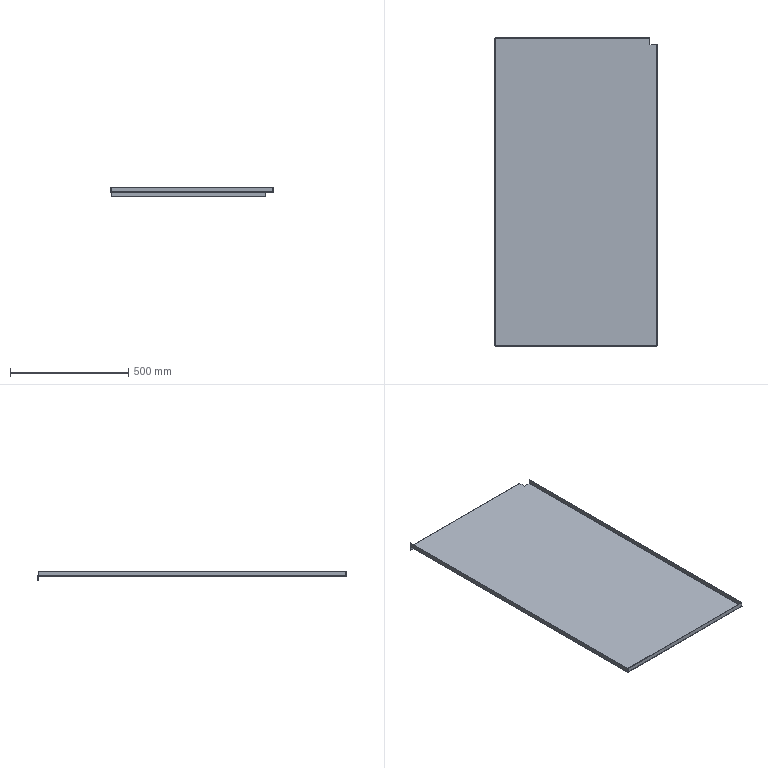Part | SolidWorks | 1 solid | 40 faces | box 685.001 x 1302 x 38.5 mm | volume 1442585 mm3 | plane 28 | cylinder 8 | spline 4 | commonest cylinder face diameters 0.2 x4 3.2 x4
STEP:
#1=CARTESIAN_POINT('',(342.5,621.,0.1));
#2=VERTEX_POINT('',#1);
#3=CARTESIAN_POINT('',(342.5,621.,18.5));
#4=VERTEX_POINT('',#3);
#5=CARTESIAN_POINT('',(342.5,621.,0.));
#6=DIRECTION('',(0.,0.,1.));
#7=VECTOR('',#6,1000.);
#8=LINE('',#5,#7);
#9=EDGE_CURVE('',#2,#4,#8,.T.);
#10=ORIENTED_EDGE('',*,*,#9,.F.);
#11=CARTESIAN_POINT('',(341.,621.,0.1));
#12=VERTEX_POINT('',#11);
#13=CARTESIAN_POINT('',(342.5,621.,0.1));
#14=DIRECTION('',(-1.,0.,0.));
#15=VECTOR('',#14,1000.);
#16=LINE('',#13,#15);
#17=EDGE_CURVE('',#2,#12,#16,.T.);
#18=ORIENTED_EDGE('',*,*,#17,.T.);
#19=CARTESIAN_POINT('',(341.,621.,18.5));
#20=VERTEX_POINT('',#19);
#21=CARTESIAN_POINT('',(341.,621.,0.));
#22=DIRECTION('',(0.,0.,1.));
#23=VECTOR('',#22,1000.);
#24=LINE('',#21,#23);
#25=EDGE_CURVE('',#12,#20,#24,.T.);
#26=ORIENTED_EDGE('',*,*,#25,.T.);
#27=CARTESIAN_POINT('',(362.5,621.,18.5));
#28=DIRECTION('',(1.,0.,0.));
#29=VECTOR('',#28,1000.);
#30=LINE('',#27,#29);
#31=EDGE_CURVE('',#20,#4,#30,.T.);
#32=ORIENTED_EDGE('',*,*,#31,.T.);
#33=EDGE_LOOP('',(#10,#18,#26,#32));
#34=FACE_OUTER_BOUND('',#33,.T.);
#35=CARTESIAN_POINT('',(362.5,621.,-20.));
#36=DIRECTION('',(0.,-1.,0.));
#37=DIRECTION('',(0.,0.,-1.));
#38=AXIS2_PLACEMENT_3D('',#35,#36,#37);
#39=PLANE('',#38);
#40=ADVANCED_FACE('',(#34),#39,.F.);
#41=CARTESIAN_POINT('',(312.5,621.,0.));
#42=VERTEX_POINT('',#41);
#43=CARTESIAN_POINT('',(340.9,621.,0.));
#44=VERTEX_POINT('',#43);
#45=CARTESIAN_POINT('',(0.,621.,0.));
#46=DIRECTION('',(1.,0.,0.));
#47=VECTOR('',#46,1000.);
#48=LINE('',#45,#47);
#49=EDGE_CURVE('',#42,#44,#48,.T.);
#50=ORIENTED_EDGE('',*,*,#49,.T.);
#51=CARTESIAN_POINT('',(340.9,621.,-1.5));
#52=VERTEX_POINT('',#51);
#53=CARTESIAN_POINT('',(340.9,621.,0.));
#54=DIRECTION('',(0.,0.,-1.));
#55=VECTOR('',#54,1000.);
#56=LINE('',#53,#55);
#57=EDGE_CURVE('',#44,#52,#56,.T.);
#58=ORIENTED_EDGE('',*,*,#57,.T.);
#59=CARTESIAN_POINT('',(312.5,621.,-1.5));
#60=VERTEX_POINT('',#59);
#61=CARTESIAN_POINT('',(0.,621.,-1.5));
#62=DIRECTION('',(1.,0.,0.));
#63=VECTOR('',#62,1000.);
#64=LINE('',#61,#63);
#65=EDGE_CURVE('',#60,#52,#64,.T.);
#66=ORIENTED_EDGE('',*,*,#65,.F.);
#67=CARTESIAN_POINT('',(312.5,621.,-20.));
#68=DIRECTION('',(0.,0.,1.));
#69=VECTOR('',#68,1000.);
#70=LINE('',#67,#69);
#71=EDGE_CURVE('',#60,#42,#70,.T.);
#72=ORIENTED_EDGE('',*,*,#71,.T.);
#73=EDGE_LOOP('',(#50,#58,#66,#72));
#74=FACE_OUTER_BOUND('',#73,.T.);
#75=CARTESIAN_POINT('',(362.5,621.,-20.));
#76=DIRECTION('',(0.,-1.,0.));
#77=DIRECTION('',(0.,0.,-1.));
#78=AXIS2_PLACEMENT_3D('',#75,#76,#77);
#79=PLANE('',#78);
#80=ADVANCED_FACE('',(#74),#79,.F.);
#81=CARTESIAN_POINT('',(312.5,651.,-20.));
#82=VERTEX_POINT('',#81);
#83=CARTESIAN_POINT('',(312.5,651.,-1.6));
#84=VERTEX_POINT('',#83);
#85=CARTESIAN_POINT('',(312.5,651.,0.));
#86=DIRECTION('',(0.,0.,1.));
#87=VECTOR('',#86,1000.);
#88=LINE('',#85,#87);
#89=EDGE_CURVE('',#82,#84,#88,.T.);
#90=ORIENTED_EDGE('',*,*,#89,.T.);
#91=CARTESIAN_POINT('',(312.5,649.5,-1.6));
#92=VERTEX_POINT('',#91);
#93=CARTESIAN_POINT('',(312.5,651.,-1.6));
#94=DIRECTION('',(0.,-1.,0.));
#95=VECTOR('',#94,1000.);
#96=LINE('',#93,#95);
#97=EDGE_CURVE('',#84,#92,#96,.T.);
#98=ORIENTED_EDGE('',*,*,#97,.T.);
#99=CARTESIAN_POINT('',(312.5,649.5,-20.));
#100=VERTEX_POINT('',#99);
#101=CARTESIAN_POINT('',(312.5,649.5,0.));
#102=DIRECTION('',(0.,0.,1.));
#103=VECTOR('',#102,1000.);
#104=LINE('',#101,#103);
#105=EDGE_CURVE('',#100,#92,#104,.T.);
#106=ORIENTED_EDGE('',*,*,#105,.F.);
#107=CARTESIAN_POINT('',(312.5,621.,-20.));
#108=DIRECTION('',(0.,-1.,0.));
#109=VECTOR('',#108,1000.);
#110=LINE('',#107,#109);
#111=EDGE_CURVE('',#82,#100,#110,.T.);
#112=ORIENTED_EDGE('',*,*,#111,.F.);
#113=EDGE_LOOP('',(#90,#98,#106,#112));
#114=FACE_OUTER_BOUND('',#113,.T.);
#115=CARTESIAN_POINT('',(312.5,621.,-20.));
#116=DIRECTION('',(-1.,0.,0.));
#117=DIRECTION('',(0.,0.,1.));
#118=AXIS2_PLACEMENT_3D('',#115,#116,#117);
#119=PLANE('',#118);
#120=ADVANCED_FACE('',(#114),#119,.F.);
#121=CARTESIAN_POINT('',(312.5,649.4,-1.5));
#122=VERTEX_POINT('',#121);
#123=CARTESIAN_POINT('',(312.5,0.,-1.5));
#124=DIRECTION('',(0.,-1.,0.));
#125=VECTOR('',#124,1000.);
#126=LINE('',#123,#125);
#127=EDGE_CURVE('',#122,#60,#126,.T.);
#128=ORIENTED_EDGE('',*,*,#127,.F.);
#129=CARTESIAN_POINT('',(312.5,649.4,0.));
#130=VERTEX_POINT('',#129);
#131=CARTESIAN_POINT('',(312.5,649.4,-1.5));
#132=DIRECTION('',(0.,0.,1.));
#133=VECTOR('',#132,1000.);
#134=LINE('',#131,#133);
#135=EDGE_CURVE('',#122,#130,#134,.T.);
#136=ORIENTED_EDGE('',*,*,#135,.T.);
#137=CARTESIAN_POINT('',(312.5,0.,0.));
#138=DIRECTION('',(0.,-1.,0.));
#139=VECTOR('',#138,1000.);
#140=LINE('',#137,#139);
#141=EDGE_CURVE('',#130,#42,#140,.T.);
#142=ORIENTED_EDGE('',*,*,#141,.T.);
#143=ORIENTED_EDGE('',*,*,#71,.F.);
#144=EDGE_LOOP('',(#128,#136,#142,#143));
#145=FACE_OUTER_BOUND('',#144,.T.);
#146=CARTESIAN_POINT('',(312.5,621.,-20.));
#147=DIRECTION('',(-1.,0.,0.));
#148=DIRECTION('',(0.,0.,1.));
#149=AXIS2_PLACEMENT_3D('',#146,#147,#148);
#150=PLANE('',#149);
#151=ADVANCED_FACE('',(#145),#150,.F.);
#152=ORIENTED_EDGE('',*,*,#127,.T.);
#153=ORIENTED_EDGE('',*,*,#65,.T.);
#154=CARTESIAN_POINT('',(340.9,-649.4,-1.5));
#155=VERTEX_POINT('',#154);
#156=CARTESIAN_POINT('',(340.9,649.4,-1.5));
#157=DIRECTION('',(0.,-1.,0.));
#158=VECTOR('',#157,1000.);
#159=LINE('',#156,#158);
#160=EDGE_CURVE('',#52,#155,#159,.T.);
#161=ORIENTED_EDGE('',*,*,#160,.T.);
#162=CARTESIAN_POINT('',(-340.9,-649.4,-1.5));
#163=VERTEX_POINT('',#162);
#164=CARTESIAN_POINT('',(340.9,-649.4,-1.5));
#165=DIRECTION('',(-1.,0.,0.));
#166=VECTOR('',#165,1000.);
#167=LINE('',#164,#166);
#168=EDGE_CURVE('',#155,#163,#167,.T.);
#169=ORIENTED_EDGE('',*,*,#168,.T.);
#170=CARTESIAN_POINT('',(-340.9,649.4,-1.5));
#171=VERTEX_POINT('',#170);
#172=CARTESIAN_POINT('',(-340.9,-649.4,-1.5));
#173=DIRECTION('',(0.,1.,0.));
#174=VECTOR('',#173,1000.);
#175=LINE('',#172,#174);
#176=EDGE_CURVE('',#163,#171,#175,.T.);
#177=ORIENTED_EDGE('',*,*,#176,.T.);
#178=CARTESIAN_POINT('',(340.9,649.4,-1.5));
#179=DIRECTION('',(-1.,0.,0.));
#180=VECTOR('',#179,1000.);
#181=LINE('',#178,#180);
#182=EDGE_CURVE('',#122,#171,#181,.T.);
#183=ORIENTED_EDGE('',*,*,#182,.F.);
#184=EDGE_LOOP('',(#152,#153,#161,#169,#177,#183));
#185=FACE_OUTER_BOUND('',#184,.T.);
#186=CARTESIAN_POINT('',(0.,0.,-1.5));
#187=DIRECTION('',(0.,0.,1.));
#188=DIRECTION('',(1.,0.,0.));
#189=AXIS2_PLACEMENT_3D('',#186,#187,#188);
#190=PLANE('',#189);
#191=ADVANCED_FACE('',(#185),#190,.F.);
#192=ORIENTED_EDGE('',*,*,#49,.F.);
#193=ORIENTED_EDGE('',*,*,#141,.F.);
#194=CARTESIAN_POINT('',(-340.9,649.4,0.));
#195=VERTEX_POINT('',#194);
#196=CARTESIAN_POINT('',(340.9,649.4,0.));
#197=DIRECTION('',(-1.,0.,0.));
#198=VECTOR('',#197,1000.);
#199=LINE('',#196,#198);
#200=EDGE_CURVE('',#130,#195,#199,.T.);
#201=ORIENTED_EDGE('',*,*,#200,.T.);
#202=CARTESIAN_POINT('',(-340.9,-649.4,0.));
#203=VERTEX_POINT('',#202);
#204=CARTESIAN_POINT('',(-340.9,-649.4,0.));
#205=DIRECTION('',(0.,1.,0.));
#206=VECTOR('',#205,1000.);
#207=LINE('',#204,#206);
#208=EDGE_CURVE('',#203,#195,#207,.T.);
#209=ORIENTED_EDGE('',*,*,#208,.F.);
#210=CARTESIAN_POINT('',(340.9,-649.4,0.));
#211=VERTEX_POINT('',#210);
#212=CARTESIAN_POINT('',(340.9,-649.4,0.));
#213=DIRECTION('',(-1.,0.,0.));
#214=VECTOR('',#213,1000.);
#215=LINE('',#212,#214);
#216=EDGE_CURVE('',#211,#203,#215,.T.);
#217=ORIENTED_EDGE('',*,*,#216,.F.);
#218=CARTESIAN_POINT('',(340.9,649.4,0.));
#219=DIRECTION('',(0.,-1.,0.));
#220=VECTOR('',#219,1000.);
#221=LINE('',#218,#220);
#222=EDGE_CURVE('',#44,#211,#221,.T.);
#223=ORIENTED_EDGE('',*,*,#222,.F.);
#224=EDGE_LOOP('',(#192,#193,#201,#209,#217,#223));
#225=FACE_OUTER_BOUND('',#224,.T.);
#226=CARTESIAN_POINT('',(0.,0.,0.));
#227=DIRECTION('',(0.,0.,1.));
#228=DIRECTION('',(1.,0.,0.));
#229=AXIS2_PLACEMENT_3D('',#226,#227,#228);
#230=PLANE('',#229);
#231=ADVANCED_FACE('',(#225),#230,.T.);
#232=CARTESIAN_POINT('',(-342.5,649.4,0.1));
#233=VERTEX_POINT('',#232);
#234=CARTESIAN_POINT('',(-341.,649.4,0.1));
#235=VERTEX_POINT('',#234);
#236=CARTESIAN_POINT('',(-341.,649.4,0.1));
#237=DIRECTION('',(1.,0.,0.));
#238=VECTOR('',#237,1000.);
#239=LINE('',#236,#238);
#240=EDGE_CURVE('',#233,#235,#239,.T.);
#241=ORIENTED_EDGE('',*,*,#240,.T.);
#242=CARTESIAN_POINT('',(-340.9,649.4,0.1));
#243=DIRECTION('',(0.,1.,0.));
#244=DIRECTION('',(0.,0.,-1.));
#245=AXIS2_PLACEMENT_3D('',#242,#243,#244);
#246=CIRCLE('',#245,0.1);
#247=EDGE_CURVE('',#195,#235,#246,.T.);
#248=ORIENTED_EDGE('',*,*,#247,.F.);
#249=CARTESIAN_POINT('',(-340.9,649.4,0.));
#250=DIRECTION('',(0.,0.,-1.));
#251=VECTOR('',#250,1000.);
#252=LINE('',#249,#251);
#253=EDGE_CURVE('',#195,#171,#252,.T.);
#254=ORIENTED_EDGE('',*,*,#253,.T.);
#255=CARTESIAN_POINT('',(-340.9,649.4,0.1));
#256=DIRECTION('',(0.,1.,0.));
#257=DIRECTION('',(0.,0.,-1.));
#258=AXIS2_PLACEMENT_3D('',#255,#256,#257);
#259=CIRCLE('',#258,1.6);
#260=EDGE_CURVE('',#171,#233,#259,.T.);
#261=ORIENTED_EDGE('',*,*,#260,.T.);
#262=EDGE_LOOP('',(#241,#248,#254,#261));
#263=FACE_OUTER_BOUND('',#262,.T.);
#264=CARTESIAN_POINT('',(-340.9,649.4,0.1));
#265=DIRECTION('',(0.,1.,0.));
#266=DIRECTION('',(0.,0.,1.));
#267=AXIS2_PLACEMENT_3D('',#264,#265,#266);
#268=PLANE('',#267);
#269=ADVANCED_FACE('',(#263),#268,.T.);
#270=CARTESIAN_POINT('',(-341.,-648.793,0.1));
#271=VERTEX_POINT('',#270);
#272=CARTESIAN_POINT('',(-341.,-648.793,0.1));
#273=CARTESIAN_POINT('',(-341.,-648.894,0.07382));
#274=CARTESIAN_POINT('',(-340.989,-648.995,0.0478));
#275=CARTESIAN_POINT('',(-340.952,-649.198,0.01078));
#276=CARTESIAN_POINT('',(-340.926,-649.299,0.));
#277=CARTESIAN_POINT('',(-340.9,-649.4,0.));
#278=B_SPLINE_CURVE_WITH_KNOTS('',3,(#272,#273,#274,#275,#276,#277),.UNSPECIFIED.,.F.,.F.,(4,2,4),(0.,0.5,1.),.UNSPECIFIED.);
#279=EDGE_CURVE('',#271,#203,#278,.T.);
#280=ORIENTED_EDGE('',*,*,#279,.F.);
#281=CARTESIAN_POINT('',(-342.5,-648.793,0.1));
#282=VERTEX_POINT('',#281);
#283=CARTESIAN_POINT('',(-341.,-648.793,0.1));
#284=DIRECTION('',(1.,0.,0.));
#285=VECTOR('',#284,1000.);
#286=LINE('',#283,#285);
#287=EDGE_CURVE('',#282,#271,#286,.T.);
#288=ORIENTED_EDGE('',*,*,#287,.F.);
#289=CARTESIAN_POINT('',(-342.5,-648.793,0.1));
#290=CARTESIAN_POINT('',(-342.5,-648.844,-0.1115));
#291=CARTESIAN_POINT('',(-342.46,-648.893,-0.3151));
#292=CARTESIAN_POINT('',(-342.299,-648.995,-0.7048));
#293=CARTESIAN_POINT('',(-342.181,-649.045,-0.881));
#294=CARTESIAN_POINT('',(-341.958,-649.121,-1.105));
#295=CARTESIAN_POINT('',(-341.878,-649.147,-1.171));
#296=CARTESIAN_POINT('',(-341.704,-649.197,-1.287));
#297=CARTESIAN_POINT('',(-341.61,-649.223,-1.338));
#298=CARTESIAN_POINT('',(-341.32,-649.299,-1.458));
#299=CARTESIAN_POINT('',(-341.112,-649.349,-1.5));
#300=CARTESIAN_POINT('',(-340.9,-649.4,-1.5));
#301=B_SPLINE_CURVE_WITH_KNOTS('',3,(#289,#290,#291,#292,#293,#294,#295,#296,#297,#298,#299,#300),.UNSPECIFIED.,.F.,.F.,(4,2,2,2,2,4),(0.,0.0006399,0.00128,0.0016,0.00192,0.00256),.UNSPECIFIED.);
#302=EDGE_CURVE('',#282,#163,#301,.T.);
#303=ORIENTED_EDGE('',*,*,#302,.T.);
#304=CARTESIAN_POINT('',(-340.9,-649.4,0.));
#305=DIRECTION('',(0.,0.,-1.));
#306=VECTOR('',#305,1000.);
#307=LINE('',#304,#306);
#308=EDGE_CURVE('',#203,#163,#307,.T.);
#309=ORIENTED_EDGE('',*,*,#308,.F.);
#310=EDGE_LOOP('',(#280,#288,#303,#309));
#311=FACE_OUTER_BOUND('',#310,.T.);
#312=CARTESIAN_POINT('',(-342.515,-648.793,0.1));
#313=CARTESIAN_POINT('',(-342.515,-648.843,-0.1114));
#314=CARTESIAN_POINT('',(-342.473,-648.894,-0.3227));
#315=CARTESIAN_POINT('',(-342.311,-648.995,-0.7133));
#316=CARTESIAN_POINT('',(-342.191,-649.046,-0.8925));
#317=CARTESIAN_POINT('',(-341.892,-649.147,-1.191));
#318=CARTESIAN_POINT('',(-341.713,-649.198,-1.311));
#319=CARTESIAN_POINT('',(-341.323,-649.299,-1.473));
#320=CARTESIAN_POINT('',(-341.111,-649.349,-1.515));
#321=CARTESIAN_POINT('',(-340.9,-649.4,-1.515));
#322=CARTESIAN_POINT('',(-342.5,-648.793,0.1));
#323=CARTESIAN_POINT('',(-342.5,-648.843,-0.1095));
#324=CARTESIAN_POINT('',(-342.458,-648.894,-0.3188));
#325=CARTESIAN_POINT('',(-342.298,-648.995,-0.7058));
#326=CARTESIAN_POINT('',(-342.179,-649.046,-0.8833));
#327=CARTESIAN_POINT('',(-341.883,-649.147,-1.179));
#328=CARTESIAN_POINT('',(-341.706,-649.198,-1.298));
#329=CARTESIAN_POINT('',(-341.319,-649.299,-1.458));
#330=CARTESIAN_POINT('',(-341.109,-649.349,-1.5));
#331=CARTESIAN_POINT('',(-340.9,-649.4,-1.5));
#332=CARTESIAN_POINT('',(-341.,-648.793,0.1));
#333=CARTESIAN_POINT('',(-341.,-648.843,0.08691));
#334=CARTESIAN_POINT('',(-340.997,-648.894,0.07383));
#335=CARTESIAN_POINT('',(-340.987,-648.995,0.04964));
#336=CARTESIAN_POINT('',(-340.98,-649.046,0.03855));
#337=CARTESIAN_POINT('',(-340.961,-649.147,0.02003));
#338=CARTESIAN_POINT('',(-340.95,-649.198,0.01262));
#339=CARTESIAN_POINT('',(-340.926,-649.299,0.002603));
#340=CARTESIAN_POINT('',(-340.913,-649.349,0.));
#341=CARTESIAN_POINT('',(-340.9,-649.4,0.));
#342=B_SPLINE_SURFACE_WITH_KNOTS('',1,3,((#312,#313,#314,#315,#316,#317,#318,#319,#320,#321),(#322,#323,#324,#325,#326,#327,#328,#329,#330,#331),(#332,#333,#334,#335,#336,#337,#338,#339,#340,#341)),.UNSPECIFIED.,.F.,.F.,.F.,(2,1,2),(4,2,2,2,4),(-0.01,0.,1.),(0.,0.25,0.5,0.75,1.),.UNSPECIFIED.);
#343=ADVANCED_FACE('',(#311),#342,.F.);
#344=ORIENTED_EDGE('',*,*,#176,.F.);
#345=ORIENTED_EDGE('',*,*,#302,.F.);
#346=CARTESIAN_POINT('',(-342.5,651.,0.1));
#347=DIRECTION('',(0.,1.,0.));
#348=VECTOR('',#347,1000.);
#349=LINE('',#346,#348);
#350=EDGE_CURVE('',#282,#233,#349,.T.);
#351=ORIENTED_EDGE('',*,*,#350,.T.);
#352=ORIENTED_EDGE('',*,*,#260,.F.);
#353=EDGE_LOOP('',(#344,#345,#351,#352));
#354=FACE_OUTER_BOUND('',#353,.T.);
#355=CARTESIAN_POINT('',(-340.9,-649.4,0.1));
#356=DIRECTION('',(0.,-1.,0.));
#357=DIRECTION('',(-1.,0.,0.));
#358=AXIS2_PLACEMENT_3D('',#355,#356,#357);
#359=CYLINDRICAL_SURFACE('',#358,1.6);
#360=ADVANCED_FACE('',(#354),#359,.T.);
#361=ORIENTED_EDGE('',*,*,#208,.T.);
#362=ORIENTED_EDGE('',*,*,#247,.T.);
#363=CARTESIAN_POINT('',(-341.,651.,0.1));
#364=DIRECTION('',(0.,-1.,0.));
#365=VECTOR('',#364,1000.);
#366=LINE('',#363,#365);
#367=EDGE_CURVE('',#235,#271,#366,.T.);
#368=ORIENTED_EDGE('',*,*,#367,.T.);
#369=ORIENTED_EDGE('',*,*,#279,.T.);
#370=EDGE_LOOP('',(#361,#362,#368,#369));
#371=FACE_OUTER_BOUND('',#370,.T.);
#372=CARTESIAN_POINT('',(-340.9,-649.4,0.1));
#373=DIRECTION('',(0.,-1.,0.));
#374=DIRECTION('',(-1.,0.,0.));
#375=AXIS2_PLACEMENT_3D('',#372,#373,#374);
#376=CYLINDRICAL_SURFACE('',#375,0.1);
#377=ADVANCED_FACE('',(#371),#376,.F.);
#378=CARTESIAN_POINT('',(-342.5,649.4,18.5));
#379=VERTEX_POINT('',#378);
#380=CARTESIAN_POINT('',(-342.5,649.4,0.));
#381=DIRECTION('',(0.,0.,1.));
#382=VECTOR('',#381,1000.);
#383=LINE('',#380,#382);
#384=EDGE_CURVE('',#233,#379,#383,.T.);
#385=ORIENTED_EDGE('',*,*,#384,.T.);
#386=CARTESIAN_POINT('',(-341.,649.4,18.5));
#387=VERTEX_POINT('',#386);
#388=CARTESIAN_POINT('',(-341.,649.4,18.5));
#389=DIRECTION('',(1.,0.,0.));
#390=VECTOR('',#389,1000.);
#391=LINE('',#388,#390);
#392=EDGE_CURVE('',#379,#387,#391,.T.);
#393=ORIENTED_EDGE('',*,*,#392,.T.);
#394=CARTESIAN_POINT('',(-341.,649.4,0.));
#395=DIRECTION('',(0.,0.,1.));
#396=VECTOR('',#395,1000.);
#397=LINE('',#394,#396);
#398=EDGE_CURVE('',#235,#387,#397,.T.);
#399=ORIENTED_EDGE('',*,*,#398,.F.);
#400=ORIENTED_EDGE('',*,*,#240,.F.);
#401=EDGE_LOOP('',(#385,#393,#399,#400));
#402=FACE_OUTER_BOUND('',#401,.T.);
#403=CARTESIAN_POINT('',(-341.,649.4,0.));
#404=DIRECTION('',(0.,1.,0.));
#405=DIRECTION('',(0.,0.,1.));
#406=AXIS2_PLACEMENT_3D('',#403,#404,#405);
#407=PLANE('',#406);
#408=ADVANCED_FACE('',(#402),#407,.T.);
#409=ORIENTED_EDGE('',*,*,#350,.F.);
#410=CARTESIAN_POINT('',(-342.5,-648.793,18.5));
#411=VERTEX_POINT('',#410);
#412=CARTESIAN_POINT('',(-342.5,-648.793,0.));
#413=DIRECTION('',(0.,0.,1.));
#414=VECTOR('',#413,1000.);
#415=LINE('',#412,#414);
#416=EDGE_CURVE('',#282,#411,#415,.T.);
#417=ORIENTED_EDGE('',*,*,#416,.T.);
#418=CARTESIAN_POINT('',(-342.5,0.,18.5));
#419=DIRECTION('',(0.,1.,0.));
#420=VECTOR('',#419,1000.);
#421=LINE('',#418,#420);
#422=EDGE_CURVE('',#411,#379,#421,.T.);
#423=ORIENTED_EDGE('',*,*,#422,.T.);
#424=ORIENTED_EDGE('',*,*,#384,.F.);
#425=EDGE_LOOP('',(#409,#417,#423,#424));
#426=FACE_OUTER_BOUND('',#425,.T.);
#427=CARTESIAN_POINT('',(-342.5,0.,0.));
#428=DIRECTION('',(1.,0.,0.));
#429=DIRECTION('',(0.,0.,-1.));
#430=AXIS2_PLACEMENT_3D('',#427,#428,#429);
#431=PLANE('',#430);
#432=ADVANCED_FACE('',(#426),#431,.F.);
#433=CARTESIAN_POINT('',(-341.,-648.793,18.5));
#434=VERTEX_POINT('',#433);
#435=CARTESIAN_POINT('',(-341.,-648.793,0.));
#436=DIRECTION('',(0.,0.,1.));
#437=VECTOR('',#436,1000.);
#438=LINE('',#435,#437);
#439=EDGE_CURVE('',#271,#434,#438,.T.);
#440=ORIENTED_EDGE('',*,*,#439,.F.);
#441=ORIENTED_EDGE('',*,*,#367,.F.);
#442=ORIENTED_EDGE('',*,*,#398,.T.);
#443=CARTESIAN_POINT('',(-341.,651.,18.5));
#444=DIRECTION('',(0.,1.,0.));
#445=VECTOR('',#444,1000.);
#446=LINE('',#443,#445);
#447=EDGE_CURVE('',#434,#387,#446,.T.);
#448=ORIENTED_EDGE('',*,*,#447,.F.);
#449=EDGE_LOOP('',(#440,#441,#442,#448));
#450=FACE_OUTER_BOUND('',#449,.T.);
#451=CARTESIAN_POINT('',(-341.,0.,0.));
#452=DIRECTION('',(1.,0.,0.));
#453=DIRECTION('',(0.,0.,-1.));
#454=AXIS2_PLACEMENT_3D('',#451,#452,#453);
#455=PLANE('',#454);
#456=ADVANCED_FACE('',(#450),#455,.T.);
#457=ORIENTED_EDGE('',*,*,#422,.F.);
#458=CARTESIAN_POINT('',(-342.5,-648.793,18.5));
#459=DIRECTION('',(1.,0.,0.));
#460=VECTOR('',#459,1000.);
#461=LINE('',#458,#460);
#462=EDGE_CURVE('',#411,#434,#461,.T.);
#463=ORIENTED_EDGE('',*,*,#462,.T.);
#464=ORIENTED_EDGE('',*,*,#447,.T.);
#465=ORIENTED_EDGE('',*,*,#392,.F.);
#466=EDGE_LOOP('',(#457,#463,#464,#465));
#467=FACE_OUTER_BOUND('',#466,.T.);
#468=CARTESIAN_POINT('',(-342.5,651.,18.5));
#469=DIRECTION('',(0.,0.,-1.));
#470=DIRECTION('',(-1.,0.,0.));
#471=AXIS2_PLACEMENT_3D('',#468,#469,#470);
#472=PLANE('',#471);
#473=ADVANCED_FACE('',(#467),#472,.F.);
#474=ORIENTED_EDGE('',*,*,#462,.F.);
#475=ORIENTED_EDGE('',*,*,#416,.F.);
#476=ORIENTED_EDGE('',*,*,#287,.T.);
#477=ORIENTED_EDGE('',*,*,#439,.T.);
#478=EDGE_LOOP('',(#474,#475,#476,#477));
#479=FACE_OUTER_BOUND('',#478,.T.);
#480=CARTESIAN_POINT('',(-341.,-648.793,0.));
#481=DIRECTION('',(0.,1.,0.));
#482=DIRECTION('',(0.,0.,1.));
#483=AXIS2_PLACEMENT_3D('',#480,#481,#482);
#484=PLANE('',#483);
#485=ADVANCED_FACE('',(#479),#484,.F.);
#486=CARTESIAN_POINT('',(-340.9,651.,-1.6));
#487=VERTEX_POINT('',#486);
#488=CARTESIAN_POINT('',(-340.9,649.5,-1.6));
#489=VERTEX_POINT('',#488);
#490=CARTESIAN_POINT('',(-340.9,649.5,-1.6));
#491=DIRECTION('',(0.,-1.,0.));
#492=VECTOR('',#491,1000.);
#493=LINE('',#490,#492);
#494=EDGE_CURVE('',#487,#489,#493,.T.);
#495=ORIENTED_EDGE('',*,*,#494,.T.);
#496=CARTESIAN_POINT('',(-340.9,649.4,-1.6));
#497=DIRECTION('',(-1.,0.,0.));
#498=DIRECTION('',(0.,0.,-1.));
#499=AXIS2_PLACEMENT_3D('',#496,#497,#498);
#500=CIRCLE('',#499,0.1);
#501=EDGE_CURVE('',#171,#489,#500,.T.);
#502=ORIENTED_EDGE('',*,*,#501,.F.);
#503=ORIENTED_EDGE('',*,*,#253,.F.);
#504=CARTESIAN_POINT('',(-340.9,649.4,-1.6));
#505=DIRECTION('',(-1.,0.,0.));
#506=DIRECTION('',(0.,0.,-1.));
#507=AXIS2_PLACEMENT_3D('',#504,#505,#506);
#508=CIRCLE('',#507,1.6);
#509=EDGE_CURVE('',#195,#487,#508,.T.);
#510=ORIENTED_EDGE('',*,*,#509,.T.);
#511=EDGE_LOOP('',(#495,#502,#503,#510));
#512=FACE_OUTER_BOUND('',#511,.T.);
#513=CARTESIAN_POINT('',(-340.9,649.4,-1.6));
#514=DIRECTION('',(-1.,0.,0.));
#515=DIRECTION('',(0.,0.,1.));
#516=AXIS2_PLACEMENT_3D('',#513,#514,#515);
#517=PLANE('',#516);
#518=ADVANCED_FACE('',(#512),#517,.T.);
#519=CARTESIAN_POINT('',(312.5,649.4,-1.6));
#520=DIRECTION('',(1.,0.,0.));
#521=DIRECTION('',(0.,0.,1.));
#522=AXIS2_PLACEMENT_3D('',#519,#520,#521);
#523=CIRCLE('',#522,1.6);
#524=EDGE_CURVE('',#84,#130,#523,.T.);
#525=ORIENTED_EDGE('',*,*,#524,.F.);
#526=CARTESIAN_POINT('',(0.,651.,-1.6));
#527=DIRECTION('',(1.,0.,0.));
#528=VECTOR('',#527,1000.);
#529=LINE('',#526,#528);
#530=EDGE_CURVE('',#487,#84,#529,.T.);
#531=ORIENTED_EDGE('',*,*,#530,.F.);
#532=ORIENTED_EDGE('',*,*,#509,.F.);
#533=ORIENTED_EDGE('',*,*,#200,.F.);
#534=EDGE_LOOP('',(#525,#531,#532,#533));
#535=FACE_OUTER_BOUND('',#534,.T.);
#536=CARTESIAN_POINT('',(340.9,649.4,-1.6));
#537=DIRECTION('',(1.,0.,0.));
#538=DIRECTION('',(0.,1.,0.));
#539=AXIS2_PLACEMENT_3D('',#536,#537,#538);
#540=CYLINDRICAL_SURFACE('',#539,1.6);
#541=ADVANCED_FACE('',(#535),#540,.T.);
#542=CARTESIAN_POINT('',(-342.5,649.5,-1.6));
#543=DIRECTION('',(1.,0.,0.));
#544=VECTOR('',#543,1000.);
#545=LINE('',#542,#544);
#546=EDGE_CURVE('',#489,#92,#545,.T.);
#547=ORIENTED_EDGE('',*,*,#546,.T.);
#548=CARTESIAN_POINT('',(312.5,649.4,-1.6));
#549=DIRECTION('',(1.,0.,0.));
#550=DIRECTION('',(0.,0.,1.));
#551=AXIS2_PLACEMENT_3D('',#548,#549,#550);
#552=CIRCLE('',#551,0.1);
#553=EDGE_CURVE('',#92,#122,#552,.T.);
#554=ORIENTED_EDGE('',*,*,#553,.T.);
#555=ORIENTED_EDGE('',*,*,#182,.T.);
#556=ORIENTED_EDGE('',*,*,#501,.T.);
#557=EDGE_LOOP('',(#547,#554,#555,#556));
#558=FACE_OUTER_BOUND('',#557,.T.);
#559=CARTESIAN_POINT('',(340.9,649.4,-1.6));
#560=DIRECTION('',(1.,0.,0.));
#561=DIRECTION('',(0.,1.,0.));
#562=AXIS2_PLACEMENT_3D('',#559,#560,#561);
#563=CYLINDRICAL_SURFACE('',#562,0.1);
#564=ADVANCED_FACE('',(#558),#563,.F.);
#565=CARTESIAN_POINT('',(-340.9,649.5,-20.));
#566=VERTEX_POINT('',#565);
#567=CARTESIAN_POINT('',(-340.9,651.,-20.));
#568=VERTEX_POINT('',#567);
#569=CARTESIAN_POINT('',(-340.9,651.,-20.));
#570=DIRECTION('',(0.,1.,0.));
#571=VECTOR('',#570,1000.);
#572=LINE('',#569,#571);
#573=EDGE_CURVE('',#566,#568,#572,.T.);
#574=ORIENTED_EDGE('',*,*,#573,.F.);
#575=CARTESIAN_POINT('',(-340.9,649.5,0.));
#576=DIRECTION('',(0.,0.,-1.));
#577=VECTOR('',#576,1000.);
#578=LINE('',#575,#577);
#579=EDGE_CURVE('',#489,#566,#578,.T.);
#580=ORIENTED_EDGE('',*,*,#579,.F.);
#581=ORIENTED_EDGE('',*,*,#494,.F.);
#582=CARTESIAN_POINT('',(-340.9,651.,0.));
#583=DIRECTION('',(0.,0.,1.));
#584=VECTOR('',#583,1000.);
#585=LINE('',#582,#584);
#586=EDGE_CURVE('',#568,#487,#585,.T.);
#587=ORIENTED_EDGE('',*,*,#586,.F.);
#588=EDGE_LOOP('',(#574,#580,#581,#587));
#589=FACE_OUTER_BOUND('',#588,.T.);
#590=CARTESIAN_POINT('',(-340.9,649.5,-1.5));
#591=DIRECTION('',(-1.,0.,0.));
#592=DIRECTION('',(0.,0.,1.));
#593=AXIS2_PLACEMENT_3D('',#590,#591,#592);
#594=PLANE('',#593);
#595=ADVANCED_FACE('',(#589),#594,.T.);
#596=ORIENTED_EDGE('',*,*,#89,.F.);
#597=CARTESIAN_POINT('',(342.5,651.,-20.));
#598=DIRECTION('',(1.,0.,0.));
#599=VECTOR('',#598,1000.);
#600=LINE('',#597,#599);
#601=EDGE_CURVE('',#568,#82,#600,.T.);
#602=ORIENTED_EDGE('',*,*,#601,.F.);
#603=ORIENTED_EDGE('',*,*,#586,.T.);
#604=ORIENTED_EDGE('',*,*,#530,.T.);
#605=EDGE_LOOP('',(#596,#602,#603,#604));
#606=FACE_OUTER_BOUND('',#605,.T.);
#607=CARTESIAN_POINT('',(0.,651.,0.));
#608=DIRECTION('',(0.,1.,0.));
#609=DIRECTION('',(-1.,0.,0.));
#610=AXIS2_PLACEMENT_3D('',#607,#608,#609);
#611=PLANE('',#610);
#612=ADVANCED_FACE('',(#606),#611,.T.);
#613=CARTESIAN_POINT('',(0.,649.5,-20.));
#614=DIRECTION('',(1.,0.,0.));
#615=VECTOR('',#614,1000.);
#616=LINE('',#613,#615);
#617=EDGE_CURVE('',#566,#100,#616,.T.);
#618=ORIENTED_EDGE('',*,*,#617,.T.);
#619=ORIENTED_EDGE('',*,*,#105,.T.);
#620=ORIENTED_EDGE('',*,*,#546,.F.);
#621=ORIENTED_EDGE('',*,*,#579,.T.);
#622=EDGE_LOOP('',(#618,#619,#620,#621));
#623=FACE_OUTER_BOUND('',#622,.T.);
#624=CARTESIAN_POINT('',(0.,649.5,0.));
#625=DIRECTION('',(0.,1.,0.));
#626=DIRECTION('',(-1.,0.,0.));
#627=AXIS2_PLACEMENT_3D('',#624,#625,#626);
#628=PLANE('',#627);
#629=ADVANCED_FACE('',(#623),#628,.F.);
#630=ORIENTED_EDGE('',*,*,#111,.T.);
#631=ORIENTED_EDGE('',*,*,#617,.F.);
#632=ORIENTED_EDGE('',*,*,#573,.T.);
#633=ORIENTED_EDGE('',*,*,#601,.T.);
#634=EDGE_LOOP('',(#630,#631,#632,#633));
#635=FACE_OUTER_BOUND('',#634,.T.);
#636=CARTESIAN_POINT('',(342.5,651.,-20.));
#637=DIRECTION('',(0.,0.,-1.));
#638=DIRECTION('',(0.,1.,0.));
#639=AXIS2_PLACEMENT_3D('',#636,#637,#638);
#640=PLANE('',#639);
#641=ADVANCED_FACE('',(#635),#640,.T.);
#642=CARTESIAN_POINT('',(342.5,-648.793,0.1));
#643=VERTEX_POINT('',#642);
#644=CARTESIAN_POINT('',(341.,-648.793,0.1));
#645=VERTEX_POINT('',#644);
#646=CARTESIAN_POINT('',(341.,-648.793,0.1));
#647=DIRECTION('',(-1.,0.,0.));
#648=VECTOR('',#647,1000.);
#649=LINE('',#646,#648);
#650=EDGE_CURVE('',#643,#645,#649,.T.);
#651=ORIENTED_EDGE('',*,*,#650,.T.);
#652=CARTESIAN_POINT('',(340.9,-649.4,0.));
#653=CARTESIAN_POINT('',(340.926,-649.299,0.));
#654=CARTESIAN_POINT('',(340.952,-649.198,0.01078));
#655=CARTESIAN_POINT('',(340.989,-648.995,0.0478));
#656=CARTESIAN_POINT('',(341.,-648.894,0.07382));
#657=CARTESIAN_POINT('',(341.,-648.793,0.1));
#658=B_SPLINE_CURVE_WITH_KNOTS('',3,(#652,#653,#654,#655,#656,#657),.UNSPECIFIED.,.F.,.F.,(4,2,4),(0.,0.5,1.),.UNSPECIFIED.);
#659=EDGE_CURVE('',#211,#645,#658,.T.);
#660=ORIENTED_EDGE('',*,*,#659,.F.);
#661=CARTESIAN_POINT('',(340.9,-649.4,0.));
#662=DIRECTION('',(0.,0.,-1.));
#663=VECTOR('',#662,1000.);
#664=LINE('',#661,#663);
#665=EDGE_CURVE('',#211,#155,#664,.T.);
#666=ORIENTED_EDGE('',*,*,#665,.T.);
#667=CARTESIAN_POINT('',(340.9,-649.4,-1.5));
#668=CARTESIAN_POINT('',(341.112,-649.349,-1.5));
#669=CARTESIAN_POINT('',(341.315,-649.3,-1.46));
#670=CARTESIAN_POINT('',(341.705,-649.198,-1.299));
#671=CARTESIAN_POINT('',(341.881,-649.148,-1.181));
#672=CARTESIAN_POINT('',(342.105,-649.071,-0.9582));
#673=CARTESIAN_POINT('',(342.171,-649.046,-0.8775));
#674=CARTESIAN_POINT('',(342.287,-648.996,-0.7041));
#675=CARTESIAN_POINT('',(342.338,-648.97,-0.6103));
#676=CARTESIAN_POINT('',(342.458,-648.894,-0.32));
#677=CARTESIAN_POINT('',(342.5,-648.844,-0.1115));
#678=CARTESIAN_POINT('',(342.5,-648.793,0.1));
#679=B_SPLINE_CURVE_WITH_KNOTS('',3,(#667,#668,#669,#670,#671,#672,#673,#674,#675,#676,#677,#678),.UNSPECIFIED.,.F.,.F.,(4,2,2,2,2,4),(0.,0.0006399,0.00128,0.0016,0.00192,0.00256),.UNSPECIFIED.);
#680=EDGE_CURVE('',#155,#643,#679,.T.);
#681=ORIENTED_EDGE('',*,*,#680,.T.);
#682=EDGE_LOOP('',(#651,#660,#666,#681));
#683=FACE_OUTER_BOUND('',#682,.T.);
#684=CARTESIAN_POINT('',(340.9,-649.4,-1.515));
#685=CARTESIAN_POINT('',(341.111,-649.349,-1.515));
#686=CARTESIAN_POINT('',(341.323,-649.299,-1.473));
#687=CARTESIAN_POINT('',(341.713,-649.198,-1.311));
#688=CARTESIAN_POINT('',(341.892,-649.147,-1.191));
#689=CARTESIAN_POINT('',(342.191,-649.046,-0.8925));
#690=CARTESIAN_POINT('',(342.311,-648.995,-0.7133));
#691=CARTESIAN_POINT('',(342.473,-648.894,-0.3227));
#692=CARTESIAN_POINT('',(342.515,-648.843,-0.1114));
#693=CARTESIAN_POINT('',(342.515,-648.793,0.1));
#694=CARTESIAN_POINT('',(340.9,-649.4,-1.5));
#695=CARTESIAN_POINT('',(341.109,-649.349,-1.5));
#696=CARTESIAN_POINT('',(341.319,-649.299,-1.458));
#697=CARTESIAN_POINT('',(341.706,-649.198,-1.298));
#698=CARTESIAN_POINT('',(341.883,-649.147,-1.179));
#699=CARTESIAN_POINT('',(342.179,-649.046,-0.8833));
#700=CARTESIAN_POINT('',(342.298,-648.995,-0.7058));
#701=CARTESIAN_POINT('',(342.458,-648.894,-0.3188));
#702=CARTESIAN_POINT('',(342.5,-648.843,-0.1095));
#703=CARTESIAN_POINT('',(342.5,-648.793,0.1));
#704=CARTESIAN_POINT('',(340.9,-649.4,0.));
#705=CARTESIAN_POINT('',(340.913,-649.349,0.));
#706=CARTESIAN_POINT('',(340.926,-649.299,0.002603));
#707=CARTESIAN_POINT('',(340.95,-649.198,0.01262));
#708=CARTESIAN_POINT('',(340.961,-649.147,0.02003));
#709=CARTESIAN_POINT('',(340.98,-649.046,0.03855));
#710=CARTESIAN_POINT('',(340.987,-648.995,0.04964));
#711=CARTESIAN_POINT('',(340.997,-648.894,0.07383));
#712=CARTESIAN_POINT('',(341.,-648.843,0.08691));
#713=CARTESIAN_POINT('',(341.,-648.793,0.1));
#714=B_SPLINE_SURFACE_WITH_KNOTS('',1,3,((#684,#685,#686,#687,#688,#689,#690,#691,#692,#693),(#694,#695,#696,#697,#698,#699,#700,#701,#702,#703),(#704,#705,#706,#707,#708,#709,#710,#711,#712,#713)),.UNSPECIFIED.,.F.,.F.,.F.,(2,1,2),(4,2,2,2,4),(-0.01,0.,1.),(0.,0.25,0.5,0.75,1.),.UNSPECIFIED.);
#715=ADVANCED_FACE('',(#683),#714,.F.);
#716=CARTESIAN_POINT('',(340.9,621.,0.1));
#717=DIRECTION('',(0.,1.,0.));
#718=DIRECTION('',(0.,0.,-1.));
#719=AXIS2_PLACEMENT_3D('',#716,#717,#718);
#720=CIRCLE('',#719,1.6);
#721=EDGE_CURVE('',#2,#52,#720,.T.);
#722=ORIENTED_EDGE('',*,*,#721,.F.);
#723=CARTESIAN_POINT('',(342.5,-651.,0.1));
#724=DIRECTION('',(0.,-1.,0.));
#725=VECTOR('',#724,1000.);
#726=LINE('',#723,#725);
#727=EDGE_CURVE('',#2,#643,#726,.T.);
#728=ORIENTED_EDGE('',*,*,#727,.T.);
#729=ORIENTED_EDGE('',*,*,#680,.F.);
#730=ORIENTED_EDGE('',*,*,#160,.F.);
#731=EDGE_LOOP('',(#722,#728,#729,#730));
#732=FACE_OUTER_BOUND('',#731,.T.);
#733=CARTESIAN_POINT('',(340.9,649.4,0.1));
#734=DIRECTION('',(0.,1.,0.));
#735=DIRECTION('',(1.,0.,0.));
#736=AXIS2_PLACEMENT_3D('',#733,#734,#735);
#737=CYLINDRICAL_SURFACE('',#736,1.6);
#738=ADVANCED_FACE('',(#732),#737,.T.);
#739=CARTESIAN_POINT('',(341.,-651.,0.1));
#740=DIRECTION('',(0.,1.,0.));
#741=VECTOR('',#740,1000.);
#742=LINE('',#739,#741);
#743=EDGE_CURVE('',#645,#12,#742,.T.);
#744=ORIENTED_EDGE('',*,*,#743,.T.);
#745=CARTESIAN_POINT('',(340.9,621.,0.1));
#746=DIRECTION('',(0.,1.,0.));
#747=DIRECTION('',(0.,0.,-1.));
#748=AXIS2_PLACEMENT_3D('',#745,#746,#747);
#749=CIRCLE('',#748,0.1);
#750=EDGE_CURVE('',#12,#44,#749,.T.);
#751=ORIENTED_EDGE('',*,*,#750,.T.);
#752=ORIENTED_EDGE('',*,*,#222,.T.);
#753=ORIENTED_EDGE('',*,*,#659,.T.);
#754=EDGE_LOOP('',(#744,#751,#752,#753));
#755=FACE_OUTER_BOUND('',#754,.T.);
#756=CARTESIAN_POINT('',(340.9,649.4,0.1));
#757=DIRECTION('',(0.,1.,0.));
#758=DIRECTION('',(1.,0.,0.));
#759=AXIS2_PLACEMENT_3D('',#756,#757,#758);
#760=CYLINDRICAL_SURFACE('',#759,0.1);
#761=ADVANCED_FACE('',(#755),#760,.F.);
#762=CARTESIAN_POINT('',(342.5,-648.793,18.5));
#763=VERTEX_POINT('',#762);
#764=CARTESIAN_POINT('',(342.5,-648.793,0.));
#765=DIRECTION('',(0.,0.,1.));
#766=VECTOR('',#765,1000.);
#767=LINE('',#764,#766);
#768=EDGE_CURVE('',#643,#763,#767,.T.);
#769=ORIENTED_EDGE('',*,*,#768,.T.);
#770=CARTESIAN_POINT('',(341.,-648.793,18.5));
#771=VERTEX_POINT('',#770);
#772=CARTESIAN_POINT('',(341.,-648.793,18.5));
#773=DIRECTION('',(-1.,0.,0.));
#774=VECTOR('',#773,1000.);
#775=LINE('',#772,#774);
#776=EDGE_CURVE('',#763,#771,#775,.T.);
#777=ORIENTED_EDGE('',*,*,#776,.T.);
#778=CARTESIAN_POINT('',(341.,-648.793,0.));
#779=DIRECTION('',(0.,0.,1.));
#780=VECTOR('',#779,1000.);
#781=LINE('',#778,#780);
#782=EDGE_CURVE('',#645,#771,#781,.T.);
#783=ORIENTED_EDGE('',*,*,#782,.F.);
#784=ORIENTED_EDGE('',*,*,#650,.F.);
#785=EDGE_LOOP('',(#769,#777,#783,#784));
#786=FACE_OUTER_BOUND('',#785,.T.);
#787=CARTESIAN_POINT('',(341.,-648.793,0.));
#788=DIRECTION('',(0.,-1.,0.));
#789=DIRECTION('',(0.,0.,-1.));
#790=AXIS2_PLACEMENT_3D('',#787,#788,#789);
#791=PLANE('',#790);
#792=ADVANCED_FACE('',(#786),#791,.T.);
#793=ORIENTED_EDGE('',*,*,#727,.F.);
#794=ORIENTED_EDGE('',*,*,#9,.T.);
#795=CARTESIAN_POINT('',(342.5,0.,18.5));
#796=DIRECTION('',(0.,-1.,0.));
#797=VECTOR('',#796,1000.);
#798=LINE('',#795,#797);
#799=EDGE_CURVE('',#4,#763,#798,.T.);
#800=ORIENTED_EDGE('',*,*,#799,.T.);
#801=ORIENTED_EDGE('',*,*,#768,.F.);
#802=EDGE_LOOP('',(#793,#794,#800,#801));
#803=FACE_OUTER_BOUND('',#802,.T.);
#804=CARTESIAN_POINT('',(342.5,0.,0.));
#805=DIRECTION('',(-1.,0.,0.));
#806=DIRECTION('',(0.,0.,1.));
#807=AXIS2_PLACEMENT_3D('',#804,#805,#806);
#808=PLANE('',#807);
#809=ADVANCED_FACE('',(#803),#808,.F.);
#810=ORIENTED_EDGE('',*,*,#25,.F.);
#811=ORIENTED_EDGE('',*,*,#743,.F.);
#812=ORIENTED_EDGE('',*,*,#782,.T.);
#813=CARTESIAN_POINT('',(341.,-651.,18.5));
#814=DIRECTION('',(0.,-1.,0.));
#815=VECTOR('',#814,1000.);
#816=LINE('',#813,#815);
#817=EDGE_CURVE('',#20,#771,#816,.T.);
#818=ORIENTED_EDGE('',*,*,#817,.F.);
#819=EDGE_LOOP('',(#810,#811,#812,#818));
#820=FACE_OUTER_BOUND('',#819,.T.);
#821=CARTESIAN_POINT('',(341.,0.,0.));
#822=DIRECTION('',(-1.,0.,0.));
#823=DIRECTION('',(0.,0.,1.));
#824=AXIS2_PLACEMENT_3D('',#821,#822,#823);
#825=PLANE('',#824);
#826=ADVANCED_FACE('',(#820),#825,.T.);
#827=ORIENTED_EDGE('',*,*,#799,.F.);
#828=ORIENTED_EDGE('',*,*,#31,.F.);
#829=ORIENTED_EDGE('',*,*,#817,.T.);
#830=ORIENTED_EDGE('',*,*,#776,.F.);
#831=EDGE_LOOP('',(#827,#828,#829,#830));
#832=FACE_OUTER_BOUND('',#831,.T.);
#833=CARTESIAN_POINT('',(342.5,-651.,18.5));
#834=DIRECTION('',(0.,0.,-1.));
#835=DIRECTION('',(-1.,0.,0.));
#836=AXIS2_PLACEMENT_3D('',#833,#834,#835);
#837=PLANE('',#836);
#838=ADVANCED_FACE('',(#832),#837,.F.);
#839=CARTESIAN_POINT('',(-340.293,-651.,0.1));
#840=VERTEX_POINT('',#839);
#841=CARTESIAN_POINT('',(-340.293,-649.5,0.1));
#842=VERTEX_POINT('',#841);
#843=CARTESIAN_POINT('',(-340.293,-649.5,0.1));
#844=DIRECTION('',(0.,1.,0.));
#845=VECTOR('',#844,1000.);
#846=LINE('',#843,#845);
#847=EDGE_CURVE('',#840,#842,#846,.T.);
#848=ORIENTED_EDGE('',*,*,#847,.T.);
#849=CARTESIAN_POINT('',(-340.9,-649.4,0.));
#850=CARTESIAN_POINT('',(-340.799,-649.426,0.));
#851=CARTESIAN_POINT('',(-340.698,-649.452,0.01078));
#852=CARTESIAN_POINT('',(-340.495,-649.489,0.0478));
#853=CARTESIAN_POINT('',(-340.394,-649.5,0.07382));
#854=CARTESIAN_POINT('',(-340.293,-649.5,0.1));
#855=B_SPLINE_CURVE_WITH_KNOTS('',3,(#849,#850,#851,#852,#853,#854),.UNSPECIFIED.,.F.,.F.,(4,2,4),(0.,0.5,1.),.UNSPECIFIED.);
#856=EDGE_CURVE('',#203,#842,#855,.T.);
#857=ORIENTED_EDGE('',*,*,#856,.F.);
#858=ORIENTED_EDGE('',*,*,#308,.T.);
#859=CARTESIAN_POINT('',(-340.9,-649.4,-1.5));
#860=CARTESIAN_POINT('',(-340.849,-649.612,-1.5));
#861=CARTESIAN_POINT('',(-340.8,-649.815,-1.46));
#862=CARTESIAN_POINT('',(-340.698,-650.205,-1.299));
#863=CARTESIAN_POINT('',(-340.648,-650.381,-1.181));
#864=CARTESIAN_POINT('',(-340.571,-650.605,-0.9582));
#865=CARTESIAN_POINT('',(-340.546,-650.671,-0.8775));
#866=CARTESIAN_POINT('',(-340.496,-650.787,-0.7041));
#867=CARTESIAN_POINT('',(-340.47,-650.838,-0.6103));
#868=CARTESIAN_POINT('',(-340.394,-650.958,-0.32));
#869=CARTESIAN_POINT('',(-340.344,-651.,-0.1115));
#870=CARTESIAN_POINT('',(-340.293,-651.,0.1));
#871=B_SPLINE_CURVE_WITH_KNOTS('',3,(#859,#860,#861,#862,#863,#864,#865,#866,#867,#868,#869,#870),.UNSPECIFIED.,.F.,.F.,(4,2,2,2,2,4),(0.,0.0006399,0.00128,0.0016,0.00192,0.00256),.UNSPECIFIED.);
#872=EDGE_CURVE('',#163,#840,#871,.T.);
#873=ORIENTED_EDGE('',*,*,#872,.T.);
#874=EDGE_LOOP('',(#848,#857,#858,#873));
#875=FACE_OUTER_BOUND('',#874,.T.);
#876=CARTESIAN_POINT('',(-340.9,-649.4,-1.515));
#877=CARTESIAN_POINT('',(-340.849,-649.611,-1.515));
#878=CARTESIAN_POINT('',(-340.799,-649.823,-1.473));
#879=CARTESIAN_POINT('',(-340.698,-650.213,-1.311));
#880=CARTESIAN_POINT('',(-340.647,-650.392,-1.191));
#881=CARTESIAN_POINT('',(-340.546,-650.691,-0.8925));
#882=CARTESIAN_POINT('',(-340.495,-650.811,-0.7133));
#883=CARTESIAN_POINT('',(-340.394,-650.973,-0.3227));
#884=CARTESIAN_POINT('',(-340.343,-651.015,-0.1114));
#885=CARTESIAN_POINT('',(-340.293,-651.015,0.1));
#886=CARTESIAN_POINT('',(-340.9,-649.4,-1.5));
#887=CARTESIAN_POINT('',(-340.849,-649.609,-1.5));
#888=CARTESIAN_POINT('',(-340.799,-649.819,-1.458));
#889=CARTESIAN_POINT('',(-340.698,-650.206,-1.298));
#890=CARTESIAN_POINT('',(-340.647,-650.383,-1.179));
#891=CARTESIAN_POINT('',(-340.546,-650.679,-0.8833));
#892=CARTESIAN_POINT('',(-340.495,-650.798,-0.7058));
#893=CARTESIAN_POINT('',(-340.394,-650.958,-0.3188));
#894=CARTESIAN_POINT('',(-340.343,-651.,-0.1095));
#895=CARTESIAN_POINT('',(-340.293,-651.,0.1));
#896=CARTESIAN_POINT('',(-340.9,-649.4,0.));
#897=CARTESIAN_POINT('',(-340.849,-649.413,0.));
#898=CARTESIAN_POINT('',(-340.799,-649.426,0.002603));
#899=CARTESIAN_POINT('',(-340.698,-649.45,0.01262));
#900=CARTESIAN_POINT('',(-340.647,-649.461,0.02003));
#901=CARTESIAN_POINT('',(-340.546,-649.48,0.03855));
#902=CARTESIAN_POINT('',(-340.495,-649.487,0.04964));
#903=CARTESIAN_POINT('',(-340.394,-649.497,0.07383));
#904=CARTESIAN_POINT('',(-340.343,-649.5,0.08691));
#905=CARTESIAN_POINT('',(-340.293,-649.5,0.1));
#906=B_SPLINE_SURFACE_WITH_KNOTS('',1,3,((#876,#877,#878,#879,#880,#881,#882,#883,#884,#885),(#886,#887,#888,#889,#890,#891,#892,#893,#894,#895),(#896,#897,#898,#899,#900,#901,#902,#903,#904,#905)),.UNSPECIFIED.,.F.,.F.,.F.,(2,1,2),(4,2,2,2,4),(-0.01,0.,1.),(0.,0.25,0.5,0.75,1.),.UNSPECIFIED.);
#907=ADVANCED_FACE('',(#875),#906,.F.);
#908=CARTESIAN_POINT('',(340.293,-649.5,0.1));
#909=VERTEX_POINT('',#908);
#910=CARTESIAN_POINT('',(340.293,-649.5,0.1));
#911=CARTESIAN_POINT('',(340.394,-649.5,0.07382));
#912=CARTESIAN_POINT('',(340.495,-649.489,0.0478));
#913=CARTESIAN_POINT('',(340.698,-649.452,0.01078));
#914=CARTESIAN_POINT('',(340.799,-649.426,0.));
#915=CARTESIAN_POINT('',(340.9,-649.4,0.));
#916=B_SPLINE_CURVE_WITH_KNOTS('',3,(#910,#911,#912,#913,#914,#915),.UNSPECIFIED.,.F.,.F.,(4,2,4),(0.,0.5,1.),.UNSPECIFIED.);
#917=EDGE_CURVE('',#909,#211,#916,.T.);
#918=ORIENTED_EDGE('',*,*,#917,.F.);
#919=CARTESIAN_POINT('',(340.293,-651.,0.1));
#920=VERTEX_POINT('',#919);
#921=CARTESIAN_POINT('',(340.293,-649.5,0.1));
#922=DIRECTION('',(0.,1.,0.));
#923=VECTOR('',#922,1000.);
#924=LINE('',#921,#923);
#925=EDGE_CURVE('',#920,#909,#924,.T.);
#926=ORIENTED_EDGE('',*,*,#925,.F.);
#927=CARTESIAN_POINT('',(340.293,-651.,0.1));
#928=CARTESIAN_POINT('',(340.344,-651.,-0.1115));
#929=CARTESIAN_POINT('',(340.393,-650.96,-0.3151));
#930=CARTESIAN_POINT('',(340.495,-650.799,-0.7048));
#931=CARTESIAN_POINT('',(340.545,-650.681,-0.881));
#932=CARTESIAN_POINT('',(340.621,-650.458,-1.105));
#933=CARTESIAN_POINT('',(340.647,-650.378,-1.171));
#934=CARTESIAN_POINT('',(340.697,-650.204,-1.287));
#935=CARTESIAN_POINT('',(340.723,-650.11,-1.338));
#936=CARTESIAN_POINT('',(340.799,-649.82,-1.458));
#937=CARTESIAN_POINT('',(340.849,-649.612,-1.5));
#938=CARTESIAN_POINT('',(340.9,-649.4,-1.5));
#939=B_SPLINE_CURVE_WITH_KNOTS('',3,(#927,#928,#929,#930,#931,#932,#933,#934,#935,#936,#937,#938),.UNSPECIFIED.,.F.,.F.,(4,2,2,2,2,4),(0.,0.0006399,0.00128,0.0016,0.00192,0.00256),.UNSPECIFIED.);
#940=EDGE_CURVE('',#920,#155,#939,.T.);
#941=ORIENTED_EDGE('',*,*,#940,.T.);
#942=ORIENTED_EDGE('',*,*,#665,.F.);
#943=EDGE_LOOP('',(#918,#926,#941,#942));
#944=FACE_OUTER_BOUND('',#943,.T.);
#945=CARTESIAN_POINT('',(340.293,-651.015,0.1));
#946=CARTESIAN_POINT('',(340.343,-651.015,-0.1114));
#947=CARTESIAN_POINT('',(340.394,-650.973,-0.3227));
#948=CARTESIAN_POINT('',(340.495,-650.811,-0.7133));
#949=CARTESIAN_POINT('',(340.546,-650.691,-0.8925));
#950=CARTESIAN_POINT('',(340.647,-650.392,-1.191));
#951=CARTESIAN_POINT('',(340.698,-650.213,-1.311));
#952=CARTESIAN_POINT('',(340.799,-649.823,-1.473));
#953=CARTESIAN_POINT('',(340.849,-649.611,-1.515));
#954=CARTESIAN_POINT('',(340.9,-649.4,-1.515));
#955=CARTESIAN_POINT('',(340.293,-651.,0.1));
#956=CARTESIAN_POINT('',(340.343,-651.,-0.1095));
#957=CARTESIAN_POINT('',(340.394,-650.958,-0.3188));
#958=CARTESIAN_POINT('',(340.495,-650.798,-0.7058));
#959=CARTESIAN_POINT('',(340.546,-650.679,-0.8833));
#960=CARTESIAN_POINT('',(340.647,-650.383,-1.179));
#961=CARTESIAN_POINT('',(340.698,-650.206,-1.298));
#962=CARTESIAN_POINT('',(340.799,-649.819,-1.458));
#963=CARTESIAN_POINT('',(340.849,-649.609,-1.5));
#964=CARTESIAN_POINT('',(340.9,-649.4,-1.5));
#965=CARTESIAN_POINT('',(340.293,-649.5,0.1));
#966=CARTESIAN_POINT('',(340.343,-649.5,0.08691));
#967=CARTESIAN_POINT('',(340.394,-649.497,0.07383));
#968=CARTESIAN_POINT('',(340.495,-649.487,0.04964));
#969=CARTESIAN_POINT('',(340.546,-649.48,0.03855));
#970=CARTESIAN_POINT('',(340.647,-649.461,0.02003));
#971=CARTESIAN_POINT('',(340.698,-649.45,0.01262));
#972=CARTESIAN_POINT('',(340.799,-649.426,0.002603));
#973=CARTESIAN_POINT('',(340.849,-649.413,0.));
#974=CARTESIAN_POINT('',(340.9,-649.4,0.));
#975=B_SPLINE_SURFACE_WITH_KNOTS('',1,3,((#945,#946,#947,#948,#949,#950,#951,#952,#953,#954),(#955,#956,#957,#958,#959,#960,#961,#962,#963,#964),(#965,#966,#967,#968,#969,#970,#971,#972,#973,#974)),.UNSPECIFIED.,.F.,.F.,.F.,(2,1,2),(4,2,2,2,4),(-0.01,0.,1.),(0.,0.25,0.5,0.75,1.),.UNSPECIFIED.);
#976=ADVANCED_FACE('',(#944),#975,.F.);
#977=ORIENTED_EDGE('',*,*,#168,.F.);
#978=ORIENTED_EDGE('',*,*,#940,.F.);
#979=CARTESIAN_POINT('',(-342.5,-651.,0.1));
#980=DIRECTION('',(-1.,0.,0.));
#981=VECTOR('',#980,1000.);
#982=LINE('',#979,#981);
#983=EDGE_CURVE('',#920,#840,#982,.T.);
#984=ORIENTED_EDGE('',*,*,#983,.T.);
#985=ORIENTED_EDGE('',*,*,#872,.F.);
#986=EDGE_LOOP('',(#977,#978,#984,#985));
#987=FACE_OUTER_BOUND('',#986,.T.);
#988=CARTESIAN_POINT('',(340.9,-649.4,0.1));
#989=DIRECTION('',(1.,0.,0.));
#990=DIRECTION('',(0.,-1.,0.));
#991=AXIS2_PLACEMENT_3D('',#988,#989,#990);
#992=CYLINDRICAL_SURFACE('',#991,1.6);
#993=ADVANCED_FACE('',(#987),#992,.T.);
#994=ORIENTED_EDGE('',*,*,#216,.T.);
#995=ORIENTED_EDGE('',*,*,#856,.T.);
#996=CARTESIAN_POINT('',(-342.5,-649.5,0.1));
#997=DIRECTION('',(1.,0.,0.));
#998=VECTOR('',#997,1000.);
#999=LINE('',#996,#998);
#1000=EDGE_CURVE('',#842,#909,#999,.T.);
#1001=ORIENTED_EDGE('',*,*,#1000,.T.);
#1002=ORIENTED_EDGE('',*,*,#917,.T.);
#1003=EDGE_LOOP('',(#994,#995,#1001,#1002));
#1004=FACE_OUTER_BOUND('',#1003,.T.);
#1005=CARTESIAN_POINT('',(340.9,-649.4,0.1));
#1006=DIRECTION('',(1.,0.,0.));
#1007=DIRECTION('',(0.,-1.,0.));
#1008=AXIS2_PLACEMENT_3D('',#1005,#1006,#1007);
#1009=CYLINDRICAL_SURFACE('',#1008,0.1);
#1010=ADVANCED_FACE('',(#1004),#1009,.F.);
#1011=CARTESIAN_POINT('',(-340.293,-651.,18.5));
#1012=VERTEX_POINT('',#1011);
#1013=CARTESIAN_POINT('',(-340.293,-651.,0.));
#1014=DIRECTION('',(0.,0.,1.));
#1015=VECTOR('',#1014,1000.);
#1016=LINE('',#1013,#1015);
#1017=EDGE_CURVE('',#840,#1012,#1016,.T.);
#1018=ORIENTED_EDGE('',*,*,#1017,.T.);
#1019=CARTESIAN_POINT('',(-340.293,-649.5,18.5));
#1020=VERTEX_POINT('',#1019);
#1021=CARTESIAN_POINT('',(-340.293,-649.5,18.5));
#1022=DIRECTION('',(0.,1.,0.));
#1023=VECTOR('',#1022,1000.);
#1024=LINE('',#1021,#1023);
#1025=EDGE_CURVE('',#1012,#1020,#1024,.T.);
#1026=ORIENTED_EDGE('',*,*,#1025,.T.);
#1027=CARTESIAN_POINT('',(-340.293,-649.5,0.));
#1028=DIRECTION('',(0.,0.,1.));
#1029=VECTOR('',#1028,1000.);
#1030=LINE('',#1027,#1029);
#1031=EDGE_CURVE('',#842,#1020,#1030,.T.);
#1032=ORIENTED_EDGE('',*,*,#1031,.F.);
#1033=ORIENTED_EDGE('',*,*,#847,.F.);
#1034=EDGE_LOOP('',(#1018,#1026,#1032,#1033));
#1035=FACE_OUTER_BOUND('',#1034,.T.);
#1036=CARTESIAN_POINT('',(-340.293,-649.5,0.));
#1037=DIRECTION('',(-1.,0.,0.));
#1038=DIRECTION('',(0.,0.,1.));
#1039=AXIS2_PLACEMENT_3D('',#1036,#1037,#1038);
#1040=PLANE('',#1039);
#1041=ADVANCED_FACE('',(#1035),#1040,.T.);
#1042=ORIENTED_EDGE('',*,*,#983,.F.);
#1043=CARTESIAN_POINT('',(340.293,-651.,18.5));
#1044=VERTEX_POINT('',#1043);
#1045=CARTESIAN_POINT('',(340.293,-651.,0.));
#1046=DIRECTION('',(0.,0.,1.));
#1047=VECTOR('',#1046,1000.);
#1048=LINE('',#1045,#1047);
#1049=EDGE_CURVE('',#920,#1044,#1048,.T.);
#1050=ORIENTED_EDGE('',*,*,#1049,.T.);
#1051=CARTESIAN_POINT('',(0.,-651.,18.5));
#1052=DIRECTION('',(-1.,0.,0.));
#1053=VECTOR('',#1052,1000.);
#1054=LINE('',#1051,#1053);
#1055=EDGE_CURVE('',#1044,#1012,#1054,.T.);
#1056=ORIENTED_EDGE('',*,*,#1055,.T.);
#1057=ORIENTED_EDGE('',*,*,#1017,.F.);
#1058=EDGE_LOOP('',(#1042,#1050,#1056,#1057));
#1059=FACE_OUTER_BOUND('',#1058,.T.);
#1060=CARTESIAN_POINT('',(0.,-651.,0.));
#1061=DIRECTION('',(0.,1.,0.));
#1062=DIRECTION('',(0.,0.,1.));
#1063=AXIS2_PLACEMENT_3D('',#1060,#1061,#1062);
#1064=PLANE('',#1063);
#1065=ADVANCED_FACE('',(#1059),#1064,.F.);
#1066=CARTESIAN_POINT('',(340.293,-649.5,18.5));
#1067=VERTEX_POINT('',#1066);
#1068=CARTESIAN_POINT('',(340.293,-649.5,0.));
#1069=DIRECTION('',(0.,0.,1.));
#1070=VECTOR('',#1069,1000.);
#1071=LINE('',#1068,#1070);
#1072=EDGE_CURVE('',#909,#1067,#1071,.T.);
#1073=ORIENTED_EDGE('',*,*,#1072,.F.);
#1074=ORIENTED_EDGE('',*,*,#1000,.F.);
#1075=ORIENTED_EDGE('',*,*,#1031,.T.);
#1076=CARTESIAN_POINT('',(-342.5,-649.5,18.5));
#1077=DIRECTION('',(-1.,0.,0.));
#1078=VECTOR('',#1077,1000.);
#1079=LINE('',#1076,#1078);
#1080=EDGE_CURVE('',#1067,#1020,#1079,.T.);
#1081=ORIENTED_EDGE('',*,*,#1080,.F.);
#1082=EDGE_LOOP('',(#1073,#1074,#1075,#1081));
#1083=FACE_OUTER_BOUND('',#1082,.T.);
#1084=CARTESIAN_POINT('',(0.,-649.5,0.));
#1085=DIRECTION('',(0.,1.,0.));
#1086=DIRECTION('',(0.,0.,1.));
#1087=AXIS2_PLACEMENT_3D('',#1084,#1085,#1086);
#1088=PLANE('',#1087);
#1089=ADVANCED_FACE('',(#1083),#1088,.T.);
#1090=ORIENTED_EDGE('',*,*,#1055,.F.);
#1091=CARTESIAN_POINT('',(340.293,-651.,18.5));
#1092=DIRECTION('',(0.,1.,0.));
#1093=VECTOR('',#1092,1000.);
#1094=LINE('',#1091,#1093);
#1095=EDGE_CURVE('',#1044,#1067,#1094,.T.);
#1096=ORIENTED_EDGE('',*,*,#1095,.T.);
#1097=ORIENTED_EDGE('',*,*,#1080,.T.);
#1098=ORIENTED_EDGE('',*,*,#1025,.F.);
#1099=EDGE_LOOP('',(#1090,#1096,#1097,#1098));
#1100=FACE_OUTER_BOUND('',#1099,.T.);
#1101=CARTESIAN_POINT('',(-342.5,-651.,18.5));
#1102=DIRECTION('',(0.,0.,-1.));
#1103=DIRECTION('',(0.,1.,0.));
#1104=AXIS2_PLACEMENT_3D('',#1101,#1102,#1103);
#1105=PLANE('',#1104);
#1106=ADVANCED_FACE('',(#1100),#1105,.F.);
#1107=ORIENTED_EDGE('',*,*,#1095,.F.);
#1108=ORIENTED_EDGE('',*,*,#1049,.F.);
#1109=ORIENTED_EDGE('',*,*,#925,.T.);
#1110=ORIENTED_EDGE('',*,*,#1072,.T.);
#1111=EDGE_LOOP('',(#1107,#1108,#1109,#1110));
#1112=FACE_OUTER_BOUND('',#1111,.T.);
#1113=CARTESIAN_POINT('',(340.293,-649.5,0.));
#1114=DIRECTION('',(-1.,0.,0.));
#1115=DIRECTION('',(0.,0.,1.));
#1116=AXIS2_PLACEMENT_3D('',#1113,#1114,#1115);
#1117=PLANE('',#1116);
#1118=ADVANCED_FACE('',(#1112),#1117,.F.);
#1119=ORIENTED_EDGE('',*,*,#97,.F.);
#1120=ORIENTED_EDGE('',*,*,#524,.T.);
#1121=ORIENTED_EDGE('',*,*,#135,.F.);
#1122=ORIENTED_EDGE('',*,*,#553,.F.);
#1123=EDGE_LOOP('',(#1119,#1120,#1121,#1122));
#1124=FACE_OUTER_BOUND('',#1123,.T.);
#1125=CARTESIAN_POINT('',(312.5,621.,-20.));
#1126=DIRECTION('',(-1.,0.,0.));
#1127=DIRECTION('',(0.,0.,1.));
#1128=AXIS2_PLACEMENT_3D('',#1125,#1126,#1127);
#1129=PLANE('',#1128);
#1130=ADVANCED_FACE('',(#1124),#1129,.F.);
#1131=ORIENTED_EDGE('',*,*,#17,.F.);
#1132=ORIENTED_EDGE('',*,*,#721,.T.);
#1133=ORIENTED_EDGE('',*,*,#57,.F.);
#1134=ORIENTED_EDGE('',*,*,#750,.F.);
#1135=EDGE_LOOP('',(#1131,#1132,#1133,#1134));
#1136=FACE_OUTER_BOUND('',#1135,.T.);
#1137=CARTESIAN_POINT('',(362.5,621.,-20.));
#1138=DIRECTION('',(0.,-1.,0.));
#1139=DIRECTION('',(0.,0.,-1.));
#1140=AXIS2_PLACEMENT_3D('',#1137,#1138,#1139);
#1141=PLANE('',#1140);
#1142=ADVANCED_FACE('',(#1136),#1141,.F.);
#1143=CLOSED_SHELL('',(#40,#80,#120,#151,#191,#231,#269,#343,#360,#377,#408,#432,#456,#473,#485,#518,#541,#564,#595,#612,#629,#641,#715,#738,#761,#792,#809,#826,#838,#907,#976,#993,#1010,#1041,#1065,#1089,#1106,#1118,#1130,#1142));
#1144=MANIFOLD_SOLID_BREP('',#1143);
#1145=CARTESIAN_POINT('',(0.,0.,0.));
#1146=DIRECTION('',(0.,0.,1.));
#1147=DIRECTION('',(1.,0.,0.));
#1148=AXIS2_PLACEMENT_3D('',#1145,#1146,#1147);
#1149=(LENGTH_UNIT()NAMED_UNIT(*)SI_UNIT(.MILLI.,.METRE.));
#1150=UNCERTAINTY_MEASURE_WITH_UNIT(LENGTH_MEASURE(0.00001),#1149,'','');
#1151=(NAMED_UNIT(*)PLANE_ANGLE_UNIT()SI_UNIT($,.RADIAN.));
#1152=(NAMED_UNIT(*)SI_UNIT($,.STERADIAN.)SOLID_ANGLE_UNIT());
#1153=(GEOMETRIC_REPRESENTATION_CONTEXT(3)GLOBAL_UNCERTAINTY_ASSIGNED_CONTEXT((#1150))GLOBAL_UNIT_ASSIGNED_CONTEXT((#1149,#1151,#1152))REPRESENTATION_CONTEXT('',''));
#1154=ADVANCED_BREP_SHAPE_REPRESENTATION('',(#1144,#1148),#1153);